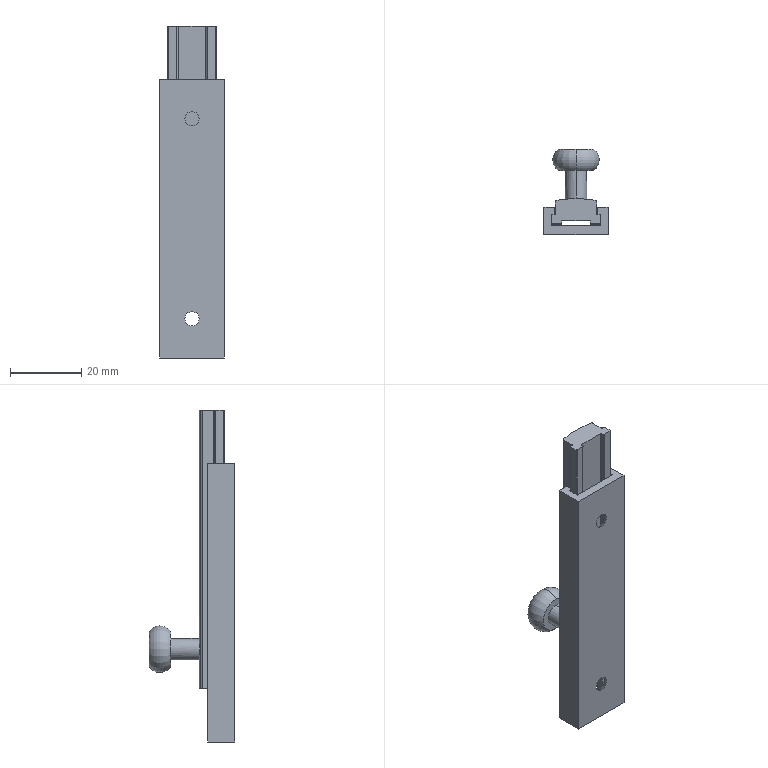Part | NX | features BREP 2 | 2 solids | 50 faces | box 18 x 24 x 93 mm | volume 12063 mm3 | plane 29 | cylinder 15 | cone 4 | torus 2 | commonest cylinder face diameters 0.5 x10 1 x2 6 x2 66.625 x1